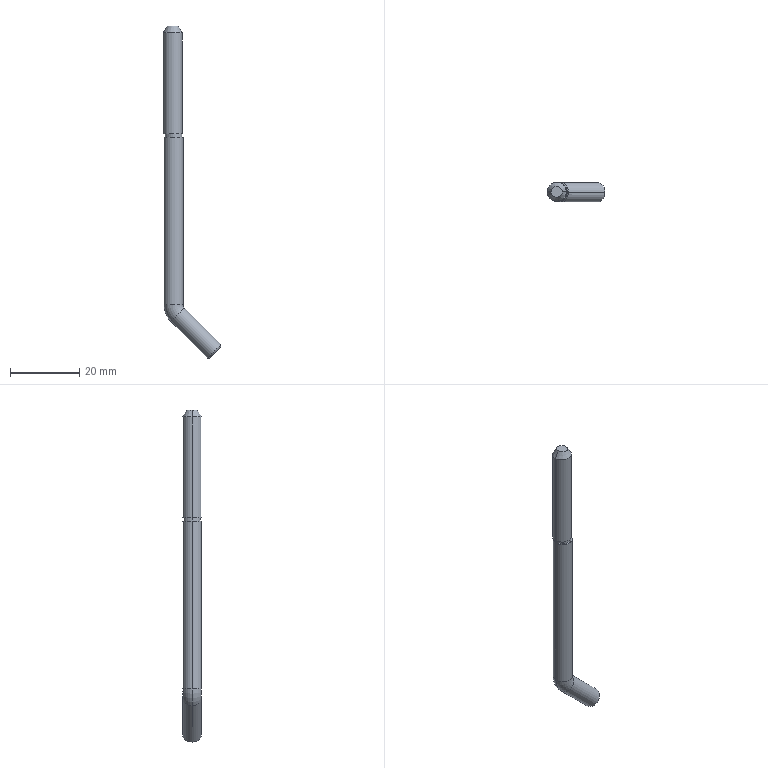Part | SolidWorks | features Chamfer 2, ICE 2, Sweep 1 | 1 solid | 18 faces | box 16.636 x 5.506 x 95.612 mm | volume 2325 mm3 | cylinder 8 | cone 4 | plane 4 | torus 2 | commonest cylinder face diameters 5.5 x4 4.8 x2 5.506 x2
STEP:
#1=CARTESIAN_POINT('',(-2.75,0.,-48.343));
#2=VERTEX_POINT('',#1);
#3=CARTESIAN_POINT('',(2.75,0.,-48.343));
#4=VERTEX_POINT('',#3);
#5=CARTESIAN_POINT('',(0.,0.,-48.343));
#6=DIRECTION('',(0.,0.,1.));
#7=DIRECTION('',(1.,0.,0.));
#8=AXIS2_PLACEMENT_3D('',#5,#6,#7);
#9=CIRCLE('',#8,2.75);
#10=EDGE_CURVE('',#2,#4,#9,.T.);
#11=ORIENTED_EDGE('',*,*,#10,.F.);
#12=CARTESIAN_POINT('',(-0.773,0.,-53.116));
#13=VERTEX_POINT('',#12);
#14=CARTESIAN_POINT('',(4.,0.,-48.343));
#15=DIRECTION('',(0.,-1.,0.));
#16=DIRECTION('',(0.,0.,-1.));
#17=AXIS2_PLACEMENT_3D('',#14,#15,#16);
#18=CIRCLE('',#17,6.75);
#19=EDGE_CURVE('',#2,#13,#18,.T.);
#20=ORIENTED_EDGE('',*,*,#19,.T.);
#21=CARTESIAN_POINT('',(3.116,0.,-49.227));
#22=VERTEX_POINT('',#21);
#23=CARTESIAN_POINT('',(1.172,0.,-51.172));
#24=DIRECTION('',(-0.7071,0.,0.7071));
#25=DIRECTION('',(0.7071,0.,0.7071));
#26=AXIS2_PLACEMENT_3D('',#23,#24,#25);
#27=CIRCLE('',#26,2.75);
#28=EDGE_CURVE('',#13,#22,#27,.T.);
#29=ORIENTED_EDGE('',*,*,#28,.T.);
#30=CARTESIAN_POINT('',(4.,0.,-48.343));
#31=DIRECTION('',(0.,-1.,0.));
#32=DIRECTION('',(0.,0.,-1.));
#33=AXIS2_PLACEMENT_3D('',#30,#31,#32);
#34=CIRCLE('',#33,1.25);
#35=EDGE_CURVE('',#4,#22,#34,.T.);
#36=ORIENTED_EDGE('',*,*,#35,.F.);
#37=EDGE_LOOP('',(#11,#20,#29,#36));
#38=FACE_OUTER_BOUND('',#37,.T.);
#39=CARTESIAN_POINT('',(4.,0.,-48.343));
#40=DIRECTION('',(0.,-1.,0.));
#41=DIRECTION('',(0.,0.,-1.));
#42=AXIS2_PLACEMENT_3D('',#39,#40,#41);
#43=TOROIDAL_SURFACE('',#42,4.,2.75);
#44=ADVANCED_FACE('',(#38),#43,.T.);
#45=CARTESIAN_POINT('',(10.43,0.,-63.612));
#46=VERTEX_POINT('',#45);
#47=CARTESIAN_POINT('',(13.612,0.,-60.43));
#48=VERTEX_POINT('',#47);
#49=CARTESIAN_POINT('',(12.021,0.,-62.021));
#50=DIRECTION('',(0.7071,0.,-0.7071));
#51=DIRECTION('',(0.7071,0.,0.7071));
#52=AXIS2_PLACEMENT_3D('',#49,#50,#51);
#53=CIRCLE('',#52,2.25);
#54=EDGE_CURVE('',#46,#48,#53,.T.);
#55=ORIENTED_EDGE('',*,*,#54,.F.);
#56=CARTESIAN_POINT('',(9.723,0.,-63.612));
#57=VERTEX_POINT('',#56);
#58=CARTESIAN_POINT('',(9.723,0.,-63.612));
#59=DIRECTION('',(-1.,0.,0.));
#60=VECTOR('',#59,1000.);
#61=LINE('',#58,#60);
#62=EDGE_CURVE('',#46,#57,#61,.T.);
#63=ORIENTED_EDGE('',*,*,#62,.T.);
#64=CARTESIAN_POINT('',(13.612,0.,-59.723));
#65=VERTEX_POINT('',#64);
#66=CARTESIAN_POINT('',(11.667,0.,-61.667));
#67=DIRECTION('',(-0.7071,0.,0.7071));
#68=DIRECTION('',(0.7071,0.,0.7071));
#69=AXIS2_PLACEMENT_3D('',#66,#67,#68);
#70=CIRCLE('',#69,2.75);
#71=EDGE_CURVE('',#65,#57,#70,.T.);
#72=ORIENTED_EDGE('',*,*,#71,.F.);
#73=CARTESIAN_POINT('',(13.612,0.,-59.723));
#74=DIRECTION('',(0.,0.,1.));
#75=VECTOR('',#74,1000.);
#76=LINE('',#73,#75);
#77=EDGE_CURVE('',#48,#65,#76,.T.);
#78=ORIENTED_EDGE('',*,*,#77,.F.);
#79=EDGE_LOOP('',(#55,#63,#72,#78));
#80=FACE_OUTER_BOUND('',#79,.T.);
#81=CARTESIAN_POINT('',(11.667,0.,-61.667));
#82=DIRECTION('',(-0.7071,0.,0.7071));
#83=DIRECTION('',(0.7071,0.,0.7071));
#84=AXIS2_PLACEMENT_3D('',#81,#82,#83);
#85=CONICAL_SURFACE('',#84,2.75,0.7854);
#86=ADVANCED_FACE('',(#80),#85,.T.);
#87=CARTESIAN_POINT('',(1.327,0.,32.));
#88=VERTEX_POINT('',#87);
#89=CARTESIAN_POINT('',(-1.87,0.,32.));
#90=VERTEX_POINT('',#89);
#91=CARTESIAN_POINT('',(-0.2714,0.,32.));
#92=DIRECTION('',(0.,0.,1.));
#93=DIRECTION('',(1.,0.,0.));
#94=AXIS2_PLACEMENT_3D('',#91,#92,#93);
#95=CIRCLE('',#94,1.598);
#96=EDGE_CURVE('',#88,#90,#95,.T.);
#97=ORIENTED_EDGE('',*,*,#96,.F.);
#98=CARTESIAN_POINT('',(2.482,0.,30.));
#99=VERTEX_POINT('',#98);
#100=CARTESIAN_POINT('',(1.327,0.,32.));
#101=DIRECTION('',(0.5,0.,-0.866));
#102=VECTOR('',#101,1000.);
#103=LINE('',#100,#102);
#104=EDGE_CURVE('',#88,#99,#103,.T.);
#105=ORIENTED_EDGE('',*,*,#104,.T.);
#106=CARTESIAN_POINT('',(-3.025,0.,30.));
#107=VERTEX_POINT('',#106);
#108=CARTESIAN_POINT('',(-0.2714,0.,30.));
#109=DIRECTION('',(0.,0.,-1.));
#110=DIRECTION('',(1.,0.,0.));
#111=AXIS2_PLACEMENT_3D('',#108,#109,#110);
#112=CIRCLE('',#111,2.753);
#113=EDGE_CURVE('',#107,#99,#112,.T.);
#114=ORIENTED_EDGE('',*,*,#113,.F.);
#115=CARTESIAN_POINT('',(-1.87,0.,32.));
#116=DIRECTION('',(-0.5,0.,-0.866));
#117=VECTOR('',#116,1000.);
#118=LINE('',#115,#117);
#119=EDGE_CURVE('',#90,#107,#118,.T.);
#120=ORIENTED_EDGE('',*,*,#119,.F.);
#121=EDGE_LOOP('',(#97,#105,#114,#120));
#122=FACE_OUTER_BOUND('',#121,.T.);
#123=CARTESIAN_POINT('',(-0.2714,0.,32.));
#124=DIRECTION('',(0.,0.,-1.));
#125=DIRECTION('',(-1.,0.,0.));
#126=AXIS2_PLACEMENT_3D('',#123,#124,#125);
#127=CONICAL_SURFACE('',#126,1.598,0.5236);
#128=ADVANCED_FACE('',(#122),#127,.T.);
#129=ORIENTED_EDGE('',*,*,#113,.T.);
#130=CARTESIAN_POINT('',(2.482,0.,1.));
#131=VERTEX_POINT('',#130);
#132=CARTESIAN_POINT('',(2.482,0.,32.));
#133=DIRECTION('',(0.,0.,-1.));
#134=VECTOR('',#133,1000.);
#135=LINE('',#132,#134);
#136=EDGE_CURVE('',#99,#131,#135,.T.);
#137=ORIENTED_EDGE('',*,*,#136,.T.);
#138=CARTESIAN_POINT('',(-3.025,0.,1.));
#139=VERTEX_POINT('',#138);
#140=CARTESIAN_POINT('',(-0.2714,0.,1.));
#141=DIRECTION('',(0.,0.,1.));
#142=DIRECTION('',(1.,0.,0.));
#143=AXIS2_PLACEMENT_3D('',#140,#141,#142);
#144=CIRCLE('',#143,2.753);
#145=EDGE_CURVE('',#131,#139,#144,.T.);
#146=ORIENTED_EDGE('',*,*,#145,.T.);
#147=CARTESIAN_POINT('',(-3.025,0.,32.));
#148=DIRECTION('',(0.,0.,-1.));
#149=VECTOR('',#148,1000.);
#150=LINE('',#147,#149);
#151=EDGE_CURVE('',#107,#139,#150,.T.);
#152=ORIENTED_EDGE('',*,*,#151,.F.);
#153=EDGE_LOOP('',(#129,#137,#146,#152));
#154=FACE_OUTER_BOUND('',#153,.T.);
#155=CARTESIAN_POINT('',(-0.2714,0.,32.));
#156=DIRECTION('',(0.,0.,-1.));
#157=DIRECTION('',(-1.,0.,0.));
#158=AXIS2_PLACEMENT_3D('',#155,#156,#157);
#159=CYLINDRICAL_SURFACE('',#158,2.753);
#160=ADVANCED_FACE('',(#154),#159,.T.);
#161=CARTESIAN_POINT('',(2.4,0.,1.));
#162=VERTEX_POINT('',#161);
#163=CARTESIAN_POINT('',(-2.4,0.,1.));
#164=VERTEX_POINT('',#163);
#165=CARTESIAN_POINT('',(0.,0.,1.));
#166=DIRECTION('',(0.,0.,1.));
#167=DIRECTION('',(1.,0.,0.));
#168=AXIS2_PLACEMENT_3D('',#165,#166,#167);
#169=CIRCLE('',#168,2.4);
#170=EDGE_CURVE('',#162,#164,#169,.T.);
#171=ORIENTED_EDGE('',*,*,#170,.F.);
#172=CARTESIAN_POINT('',(2.4,0.,0.));
#173=VERTEX_POINT('',#172);
#174=CARTESIAN_POINT('',(2.4,0.,1.));
#175=DIRECTION('',(0.,0.,-1.));
#176=VECTOR('',#175,1000.);
#177=LINE('',#174,#176);
#178=EDGE_CURVE('',#162,#173,#177,.T.);
#179=ORIENTED_EDGE('',*,*,#178,.T.);
#180=CARTESIAN_POINT('',(-2.4,0.,0.));
#181=VERTEX_POINT('',#180);
#182=CARTESIAN_POINT('',(0.,0.,0.));
#183=DIRECTION('',(0.,0.,1.));
#184=DIRECTION('',(1.,0.,0.));
#185=AXIS2_PLACEMENT_3D('',#182,#183,#184);
#186=CIRCLE('',#185,2.4);
#187=EDGE_CURVE('',#173,#181,#186,.T.);
#188=ORIENTED_EDGE('',*,*,#187,.T.);
#189=CARTESIAN_POINT('',(-2.4,0.,1.));
#190=DIRECTION('',(0.,0.,-1.));
#191=VECTOR('',#190,1000.);
#192=LINE('',#189,#191);
#193=EDGE_CURVE('',#164,#181,#192,.T.);
#194=ORIENTED_EDGE('',*,*,#193,.F.);
#195=EDGE_LOOP('',(#171,#179,#188,#194));
#196=FACE_OUTER_BOUND('',#195,.T.);
#197=CARTESIAN_POINT('',(0.,0.,1.));
#198=DIRECTION('',(0.,0.,-1.));
#199=DIRECTION('',(-1.,0.,0.));
#200=AXIS2_PLACEMENT_3D('',#197,#198,#199);
#201=CYLINDRICAL_SURFACE('',#200,2.4);
#202=ADVANCED_FACE('',(#196),#201,.T.);
#203=CARTESIAN_POINT('',(0.,0.,-48.343));
#204=DIRECTION('',(0.,0.,1.));
#205=DIRECTION('',(1.,0.,0.));
#206=AXIS2_PLACEMENT_3D('',#203,#204,#205);
#207=CIRCLE('',#206,2.75);
#208=EDGE_CURVE('',#4,#2,#207,.T.);
#209=ORIENTED_EDGE('',*,*,#208,.T.);
#210=CARTESIAN_POINT('',(-2.75,0.,0.));
#211=VERTEX_POINT('',#210);
#212=CARTESIAN_POINT('',(-2.75,0.,-48.343));
#213=DIRECTION('',(0.,0.,1.));
#214=VECTOR('',#213,1000.);
#215=LINE('',#212,#214);
#216=EDGE_CURVE('',#2,#211,#215,.T.);
#217=ORIENTED_EDGE('',*,*,#216,.T.);
#218=CARTESIAN_POINT('',(2.75,0.,0.));
#219=VERTEX_POINT('',#218);
#220=CARTESIAN_POINT('',(0.,0.,0.));
#221=DIRECTION('',(0.,0.,1.));
#222=DIRECTION('',(1.,0.,0.));
#223=AXIS2_PLACEMENT_3D('',#220,#221,#222);
#224=CIRCLE('',#223,2.75);
#225=EDGE_CURVE('',#219,#211,#224,.T.);
#226=ORIENTED_EDGE('',*,*,#225,.F.);
#227=CARTESIAN_POINT('',(2.75,0.,-48.343));
#228=DIRECTION('',(0.,0.,1.));
#229=VECTOR('',#228,1000.);
#230=LINE('',#227,#229);
#231=EDGE_CURVE('',#4,#219,#230,.T.);
#232=ORIENTED_EDGE('',*,*,#231,.F.);
#233=EDGE_LOOP('',(#209,#217,#226,#232));
#234=FACE_OUTER_BOUND('',#233,.T.);
#235=CARTESIAN_POINT('',(0.,0.,-48.343));
#236=DIRECTION('',(0.,0.,1.));
#237=DIRECTION('',(1.,0.,0.));
#238=AXIS2_PLACEMENT_3D('',#235,#236,#237);
#239=CYLINDRICAL_SURFACE('',#238,2.75);
#240=ADVANCED_FACE('',(#234),#239,.T.);
#241=CARTESIAN_POINT('',(1.172,0.,-51.172));
#242=DIRECTION('',(-0.7071,0.,0.7071));
#243=DIRECTION('',(0.7071,0.,0.7071));
#244=AXIS2_PLACEMENT_3D('',#241,#242,#243);
#245=CIRCLE('',#244,2.75);
#246=EDGE_CURVE('',#22,#13,#245,.T.);
#247=ORIENTED_EDGE('',*,*,#246,.F.);
#248=CARTESIAN_POINT('',(3.116,0.,-49.227));
#249=DIRECTION('',(0.7071,0.,-0.7071));
#250=VECTOR('',#249,1000.);
#251=LINE('',#248,#250);
#252=EDGE_CURVE('',#22,#65,#251,.T.);
#253=ORIENTED_EDGE('',*,*,#252,.T.);
#254=ORIENTED_EDGE('',*,*,#71,.T.);
#255=CARTESIAN_POINT('',(-0.773,0.,-53.116));
#256=DIRECTION('',(0.7071,0.,-0.7071));
#257=VECTOR('',#256,1000.);
#258=LINE('',#255,#257);
#259=EDGE_CURVE('',#13,#57,#258,.T.);
#260=ORIENTED_EDGE('',*,*,#259,.F.);
#261=EDGE_LOOP('',(#247,#253,#254,#260));
#262=FACE_OUTER_BOUND('',#261,.T.);
#263=CARTESIAN_POINT('',(1.172,0.,-51.172));
#264=DIRECTION('',(0.7071,0.,-0.7071));
#265=DIRECTION('',(-0.7071,0.,-0.7071));
#266=AXIS2_PLACEMENT_3D('',#263,#264,#265);
#267=CYLINDRICAL_SURFACE('',#266,2.75);
#268=ADVANCED_FACE('',(#262),#267,.T.);
#269=ORIENTED_EDGE('',*,*,#225,.T.);
#270=CARTESIAN_POINT('',(0.,0.,0.));
#271=DIRECTION('',(0.,0.,1.));
#272=DIRECTION('',(1.,0.,0.));
#273=AXIS2_PLACEMENT_3D('',#270,#271,#272);
#274=CIRCLE('',#273,2.75);
#275=EDGE_CURVE('',#211,#219,#274,.T.);
#276=ORIENTED_EDGE('',*,*,#275,.T.);
#277=EDGE_LOOP('',(#269,#276));
#278=FACE_OUTER_BOUND('',#277,.T.);
#279=CARTESIAN_POINT('',(0.,0.,0.));
#280=DIRECTION('',(0.,0.,1.));
#281=DIRECTION('',(1.,0.,0.));
#282=AXIS2_PLACEMENT_3D('',#279,#280,#281);
#283=CIRCLE('',#282,2.4);
#284=EDGE_CURVE('',#181,#173,#283,.T.);
#285=ORIENTED_EDGE('',*,*,#284,.F.);
#286=ORIENTED_EDGE('',*,*,#187,.F.);
#287=EDGE_LOOP('',(#285,#286));
#288=FACE_BOUND('',#287,.T.);
#289=CARTESIAN_POINT('',(0.,0.,0.));
#290=DIRECTION('',(0.,0.,1.));
#291=DIRECTION('',(1.,0.,0.));
#292=AXIS2_PLACEMENT_3D('',#289,#290,#291);
#293=PLANE('',#292);
#294=ADVANCED_FACE('',(#278,#288),#293,.T.);
#295=ORIENTED_EDGE('',*,*,#252,.F.);
#296=ORIENTED_EDGE('',*,*,#28,.F.);
#297=ORIENTED_EDGE('',*,*,#259,.T.);
#298=CARTESIAN_POINT('',(11.667,0.,-61.667));
#299=DIRECTION('',(-0.7071,0.,0.7071));
#300=DIRECTION('',(0.7071,0.,0.7071));
#301=AXIS2_PLACEMENT_3D('',#298,#299,#300);
#302=CIRCLE('',#301,2.75);
#303=EDGE_CURVE('',#57,#65,#302,.T.);
#304=ORIENTED_EDGE('',*,*,#303,.T.);
#305=EDGE_LOOP('',(#295,#296,#297,#304));
#306=FACE_OUTER_BOUND('',#305,.T.);
#307=CARTESIAN_POINT('',(1.172,0.,-51.172));
#308=DIRECTION('',(0.7071,0.,-0.7071));
#309=DIRECTION('',(-0.7071,0.,-0.7071));
#310=AXIS2_PLACEMENT_3D('',#307,#308,#309);
#311=CYLINDRICAL_SURFACE('',#310,2.75);
#312=ADVANCED_FACE('',(#306),#311,.T.);
#313=ORIENTED_EDGE('',*,*,#19,.F.);
#314=ORIENTED_EDGE('',*,*,#208,.F.);
#315=ORIENTED_EDGE('',*,*,#35,.T.);
#316=ORIENTED_EDGE('',*,*,#246,.T.);
#317=EDGE_LOOP('',(#313,#314,#315,#316));
#318=FACE_OUTER_BOUND('',#317,.T.);
#319=CARTESIAN_POINT('',(4.,0.,-48.343));
#320=DIRECTION('',(0.,-1.,0.));
#321=DIRECTION('',(0.,0.,-1.));
#322=AXIS2_PLACEMENT_3D('',#319,#320,#321);
#323=TOROIDAL_SURFACE('',#322,4.,2.75);
#324=ADVANCED_FACE('',(#318),#323,.T.);
#325=ORIENTED_EDGE('',*,*,#216,.F.);
#326=ORIENTED_EDGE('',*,*,#10,.T.);
#327=ORIENTED_EDGE('',*,*,#231,.T.);
#328=ORIENTED_EDGE('',*,*,#275,.F.);
#329=EDGE_LOOP('',(#325,#326,#327,#328));
#330=FACE_OUTER_BOUND('',#329,.T.);
#331=CARTESIAN_POINT('',(0.,0.,-48.343));
#332=DIRECTION('',(0.,0.,1.));
#333=DIRECTION('',(1.,0.,0.));
#334=AXIS2_PLACEMENT_3D('',#331,#332,#333);
#335=CYLINDRICAL_SURFACE('',#334,2.75);
#336=ADVANCED_FACE('',(#330),#335,.T.);
#337=CARTESIAN_POINT('',(12.021,0.,-62.021));
#338=DIRECTION('',(0.7071,0.,-0.7071));
#339=DIRECTION('',(0.7071,0.,0.7071));
#340=AXIS2_PLACEMENT_3D('',#337,#338,#339);
#341=CIRCLE('',#340,2.25);
#342=EDGE_CURVE('',#48,#46,#341,.T.);
#343=ORIENTED_EDGE('',*,*,#342,.T.);
#344=ORIENTED_EDGE('',*,*,#54,.T.);
#345=EDGE_LOOP('',(#343,#344));
#346=FACE_OUTER_BOUND('',#345,.T.);
#347=CARTESIAN_POINT('',(12.021,0.,-62.021));
#348=DIRECTION('',(-0.7071,0.,0.7071));
#349=DIRECTION('',(0.7071,0.,0.7071));
#350=AXIS2_PLACEMENT_3D('',#347,#348,#349);
#351=PLANE('',#350);
#352=ADVANCED_FACE('',(#346),#351,.F.);
#353=ORIENTED_EDGE('',*,*,#178,.F.);
#354=CARTESIAN_POINT('',(0.,0.,1.));
#355=DIRECTION('',(0.,0.,1.));
#356=DIRECTION('',(1.,0.,0.));
#357=AXIS2_PLACEMENT_3D('',#354,#355,#356);
#358=CIRCLE('',#357,2.4);
#359=EDGE_CURVE('',#164,#162,#358,.T.);
#360=ORIENTED_EDGE('',*,*,#359,.F.);
#361=ORIENTED_EDGE('',*,*,#193,.T.);
#362=ORIENTED_EDGE('',*,*,#284,.T.);
#363=EDGE_LOOP('',(#353,#360,#361,#362));
#364=FACE_OUTER_BOUND('',#363,.T.);
#365=CARTESIAN_POINT('',(0.,0.,1.));
#366=DIRECTION('',(0.,0.,-1.));
#367=DIRECTION('',(-1.,0.,0.));
#368=AXIS2_PLACEMENT_3D('',#365,#366,#367);
#369=CYLINDRICAL_SURFACE('',#368,2.4);
#370=ADVANCED_FACE('',(#364),#369,.T.);
#371=CARTESIAN_POINT('',(-0.2714,0.,1.));
#372=DIRECTION('',(0.,0.,1.));
#373=DIRECTION('',(1.,0.,0.));
#374=AXIS2_PLACEMENT_3D('',#371,#372,#373);
#375=CIRCLE('',#374,2.753);
#376=EDGE_CURVE('',#139,#131,#375,.T.);
#377=ORIENTED_EDGE('',*,*,#376,.F.);
#378=ORIENTED_EDGE('',*,*,#145,.F.);
#379=EDGE_LOOP('',(#377,#378));
#380=FACE_OUTER_BOUND('',#379,.T.);
#381=ORIENTED_EDGE('',*,*,#359,.T.);
#382=ORIENTED_EDGE('',*,*,#170,.T.);
#383=EDGE_LOOP('',(#381,#382));
#384=FACE_BOUND('',#383,.T.);
#385=CARTESIAN_POINT('',(-0.2714,0.,1.));
#386=DIRECTION('',(0.,0.,1.));
#387=DIRECTION('',(1.,0.,0.));
#388=AXIS2_PLACEMENT_3D('',#385,#386,#387);
#389=PLANE('',#388);
#390=ADVANCED_FACE('',(#380,#384),#389,.F.);
#391=ORIENTED_EDGE('',*,*,#136,.F.);
#392=CARTESIAN_POINT('',(-0.2714,0.,30.));
#393=DIRECTION('',(0.,0.,-1.));
#394=DIRECTION('',(1.,0.,0.));
#395=AXIS2_PLACEMENT_3D('',#392,#393,#394);
#396=CIRCLE('',#395,2.753);
#397=EDGE_CURVE('',#99,#107,#396,.T.);
#398=ORIENTED_EDGE('',*,*,#397,.T.);
#399=ORIENTED_EDGE('',*,*,#151,.T.);
#400=ORIENTED_EDGE('',*,*,#376,.T.);
#401=EDGE_LOOP('',(#391,#398,#399,#400));
#402=FACE_OUTER_BOUND('',#401,.T.);
#403=CARTESIAN_POINT('',(-0.2714,0.,32.));
#404=DIRECTION('',(0.,0.,-1.));
#405=DIRECTION('',(-1.,0.,0.));
#406=AXIS2_PLACEMENT_3D('',#403,#404,#405);
#407=CYLINDRICAL_SURFACE('',#406,2.753);
#408=ADVANCED_FACE('',(#402),#407,.T.);
#409=CARTESIAN_POINT('',(-0.2714,0.,32.));
#410=DIRECTION('',(0.,0.,1.));
#411=DIRECTION('',(1.,0.,0.));
#412=AXIS2_PLACEMENT_3D('',#409,#410,#411);
#413=CIRCLE('',#412,1.598);
#414=EDGE_CURVE('',#90,#88,#413,.T.);
#415=ORIENTED_EDGE('',*,*,#414,.T.);
#416=ORIENTED_EDGE('',*,*,#96,.T.);
#417=EDGE_LOOP('',(#415,#416));
#418=FACE_OUTER_BOUND('',#417,.T.);
#419=CARTESIAN_POINT('',(-0.2714,0.,32.));
#420=DIRECTION('',(0.,0.,1.));
#421=DIRECTION('',(1.,0.,0.));
#422=AXIS2_PLACEMENT_3D('',#419,#420,#421);
#423=PLANE('',#422);
#424=ADVANCED_FACE('',(#418),#423,.T.);
#425=ORIENTED_EDGE('',*,*,#104,.F.);
#426=ORIENTED_EDGE('',*,*,#414,.F.);
#427=ORIENTED_EDGE('',*,*,#119,.T.);
#428=ORIENTED_EDGE('',*,*,#397,.F.);
#429=EDGE_LOOP('',(#425,#426,#427,#428));
#430=FACE_OUTER_BOUND('',#429,.T.);
#431=CARTESIAN_POINT('',(-0.2714,0.,32.));
#432=DIRECTION('',(0.,0.,-1.));
#433=DIRECTION('',(-1.,0.,0.));
#434=AXIS2_PLACEMENT_3D('',#431,#432,#433);
#435=CONICAL_SURFACE('',#434,1.598,0.5236);
#436=ADVANCED_FACE('',(#430),#435,.T.);
#437=ORIENTED_EDGE('',*,*,#62,.F.);
#438=ORIENTED_EDGE('',*,*,#342,.F.);
#439=ORIENTED_EDGE('',*,*,#77,.T.);
#440=ORIENTED_EDGE('',*,*,#303,.F.);
#441=EDGE_LOOP('',(#437,#438,#439,#440));
#442=FACE_OUTER_BOUND('',#441,.T.);
#443=CARTESIAN_POINT('',(11.667,0.,-61.667));
#444=DIRECTION('',(-0.7071,0.,0.7071));
#445=DIRECTION('',(0.7071,0.,0.7071));
#446=AXIS2_PLACEMENT_3D('',#443,#444,#445);
#447=CONICAL_SURFACE('',#446,2.75,0.7854);
#448=ADVANCED_FACE('',(#442),#447,.T.);
#449=CLOSED_SHELL('',(#44,#86,#128,#160,#202,#240,#268,#294,#312,#324,#336,#352,#370,#390,#408,#424,#436,#448));
#450=MANIFOLD_SOLID_BREP('',#449);
#451=CARTESIAN_POINT('',(0.,0.,0.));
#452=DIRECTION('',(0.,0.,1.));
#453=DIRECTION('',(1.,0.,0.));
#454=AXIS2_PLACEMENT_3D('',#451,#452,#453);
#455=(LENGTH_UNIT()NAMED_UNIT(*)SI_UNIT(.MILLI.,.METRE.));
#456=UNCERTAINTY_MEASURE_WITH_UNIT(LENGTH_MEASURE(0.00001),#455,'','');
#457=(NAMED_UNIT(*)PLANE_ANGLE_UNIT()SI_UNIT($,.RADIAN.));
#458=(NAMED_UNIT(*)SI_UNIT($,.STERADIAN.)SOLID_ANGLE_UNIT());
#459=(GEOMETRIC_REPRESENTATION_CONTEXT(3)GLOBAL_UNCERTAINTY_ASSIGNED_CONTEXT((#456))GLOBAL_UNIT_ASSIGNED_CONTEXT((#455,#457,#458))REPRESENTATION_CONTEXT('',''));
#460=ADVANCED_BREP_SHAPE_REPRESENTATION('',(#450,#454),#459);